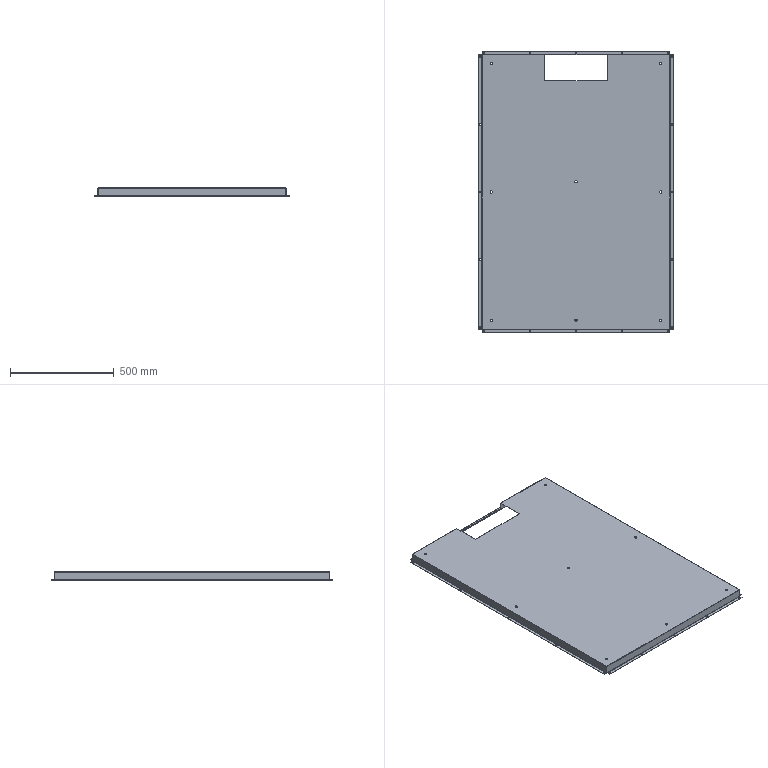Part | SolidWorks | features ICE 4, EdgeFlange 2, Cut 1, FlatPattern 1, SMBaseFlange 1, SheetMetal 1 | 1 solid | 186 faces | box 939 x 1359 x 40 mm | volume 1396732 mm3 | plane 94 | cylinder 84 | spline 8 | commonest cylinder face diameters 7 x50 11 x16 0.4 x9 2.4 x9